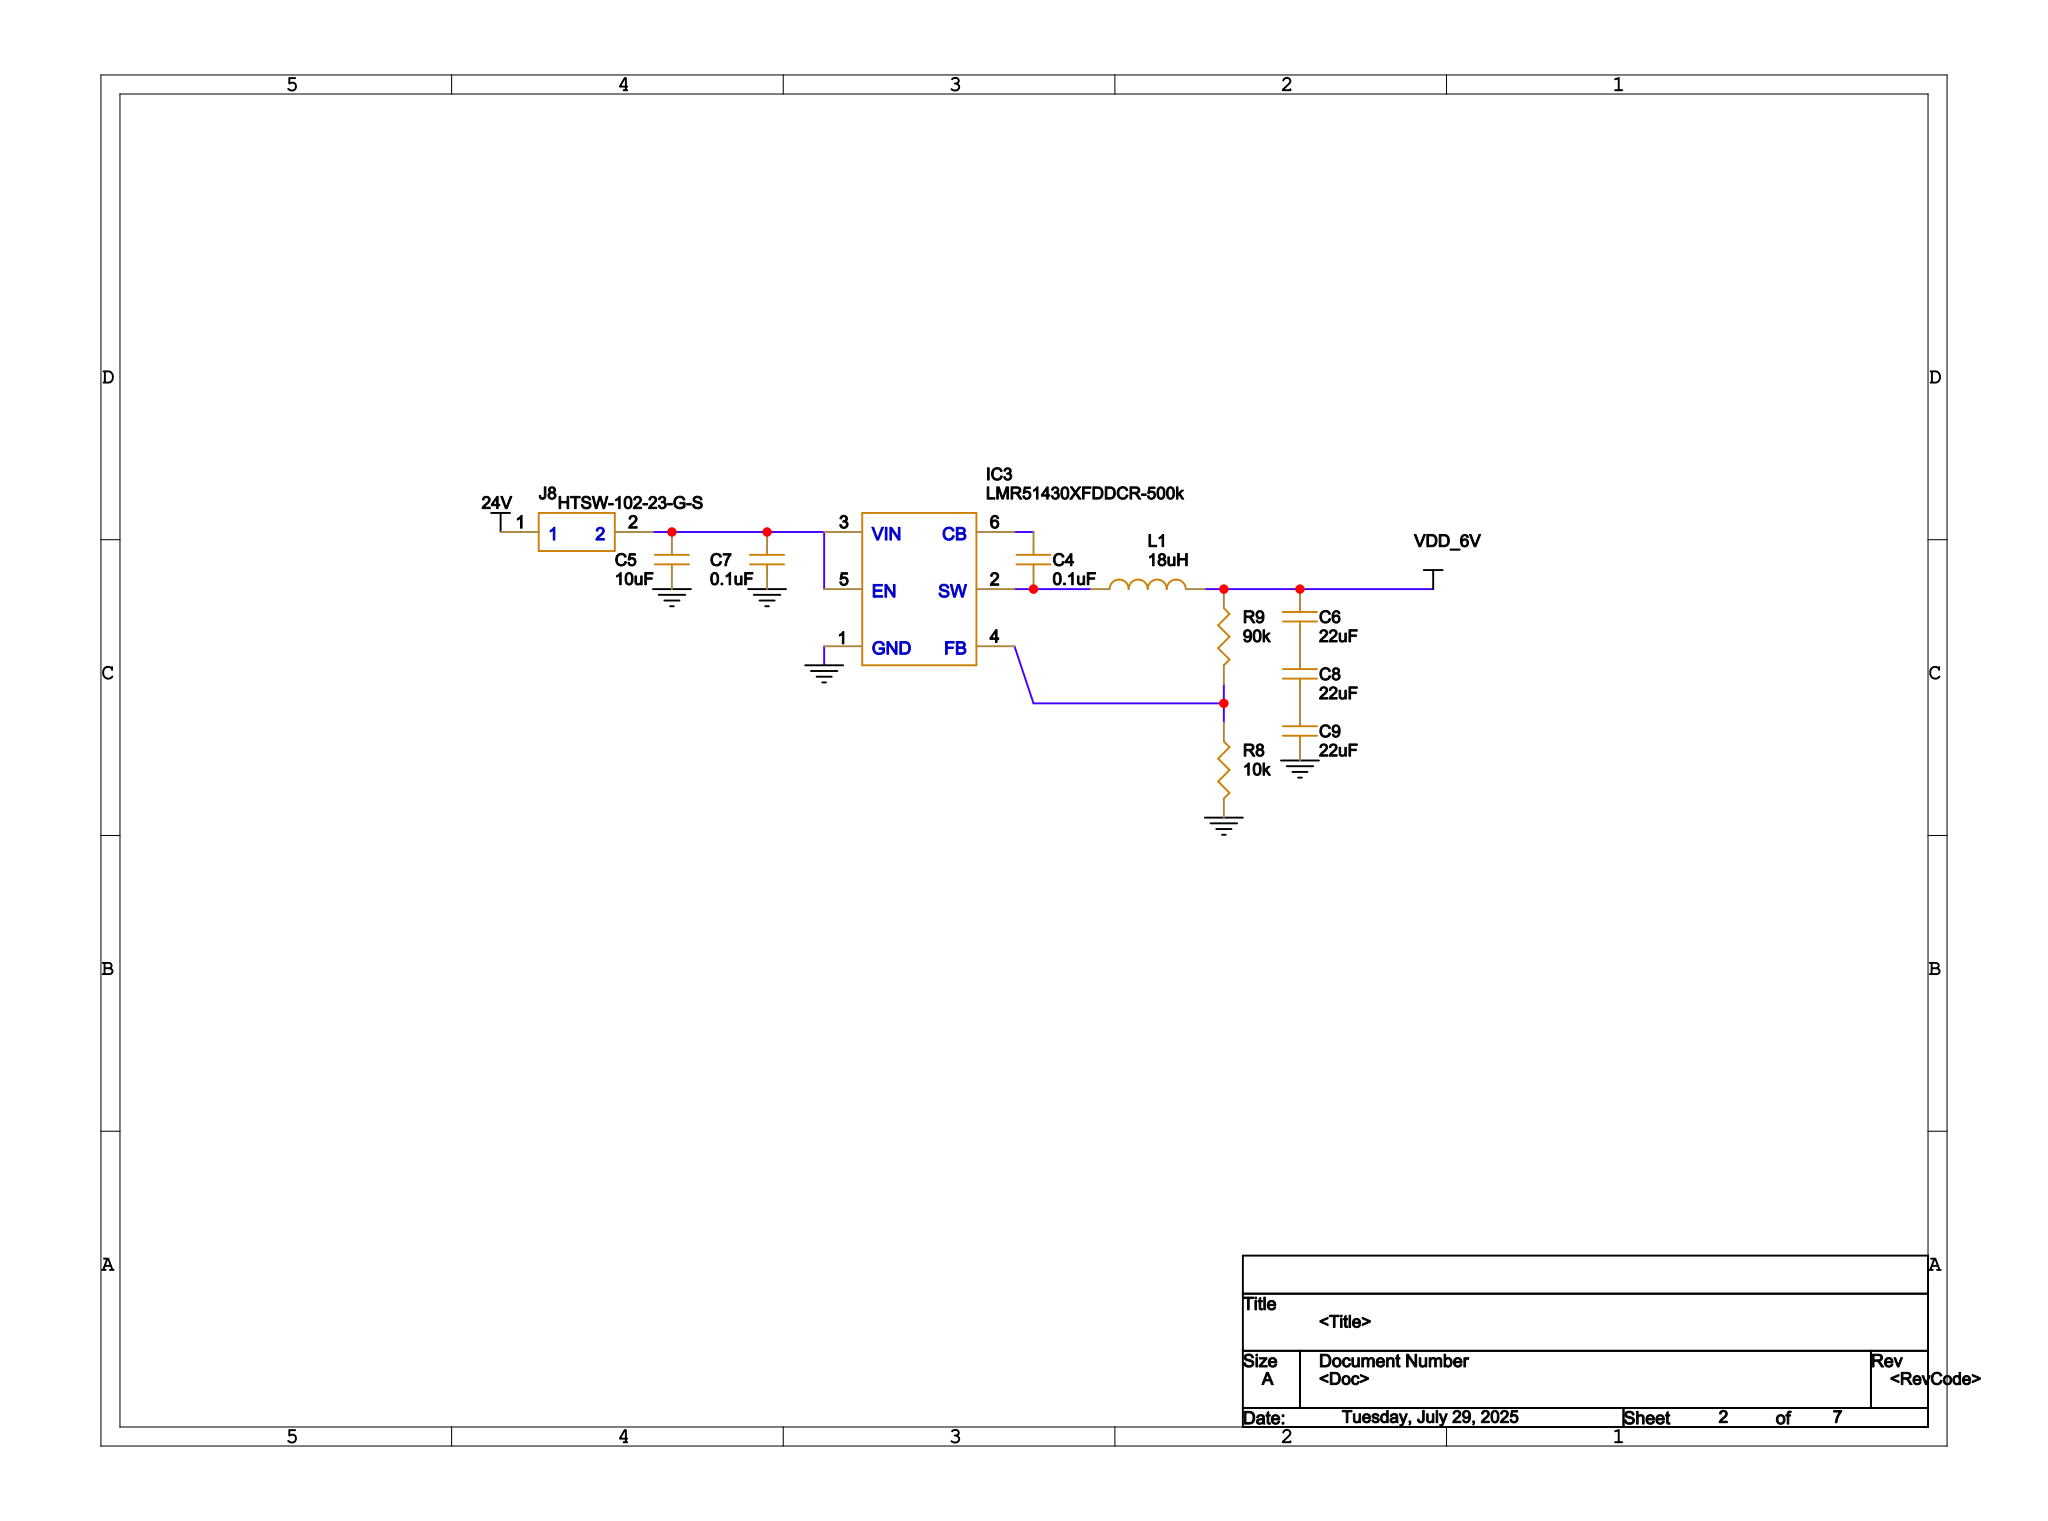Circuit board | Cadence Allegro | 93 parts | 49 nets | one sheet of the schematic
Parts on this sheet (reference | value | footprint):
C4 | 0.1uF | C0402
C5 | 10uF | C1210
C6 | 22uF | C2220
C7 | 0.1uF | C0402
C8 | 22uF | C2220
C9 | 22uF | C2220
IC3 | LMR51430XFDDCR-500k | SOT95P280X110-6N
L1 | 18uH | INDPM6868X420N
R8 | 10k | R0402
R9 | 90k | R1206
Nets of these parts (net: part-pin ...):
VDD_6V: C6-1 L1-2 R9-1
N045971: C6-2 C8-1
N048311: C8-2 C9-1
GND: C5-2 C7-2 C9-2 IC3-1 R8-2
N03630: C5-1 C7-1 IC3-3 IC3-5
N14357: IC3-4 R8-1 R9-2
N03908: C4-1 IC3-6
N04207: C4-2 IC3-2 L1-1